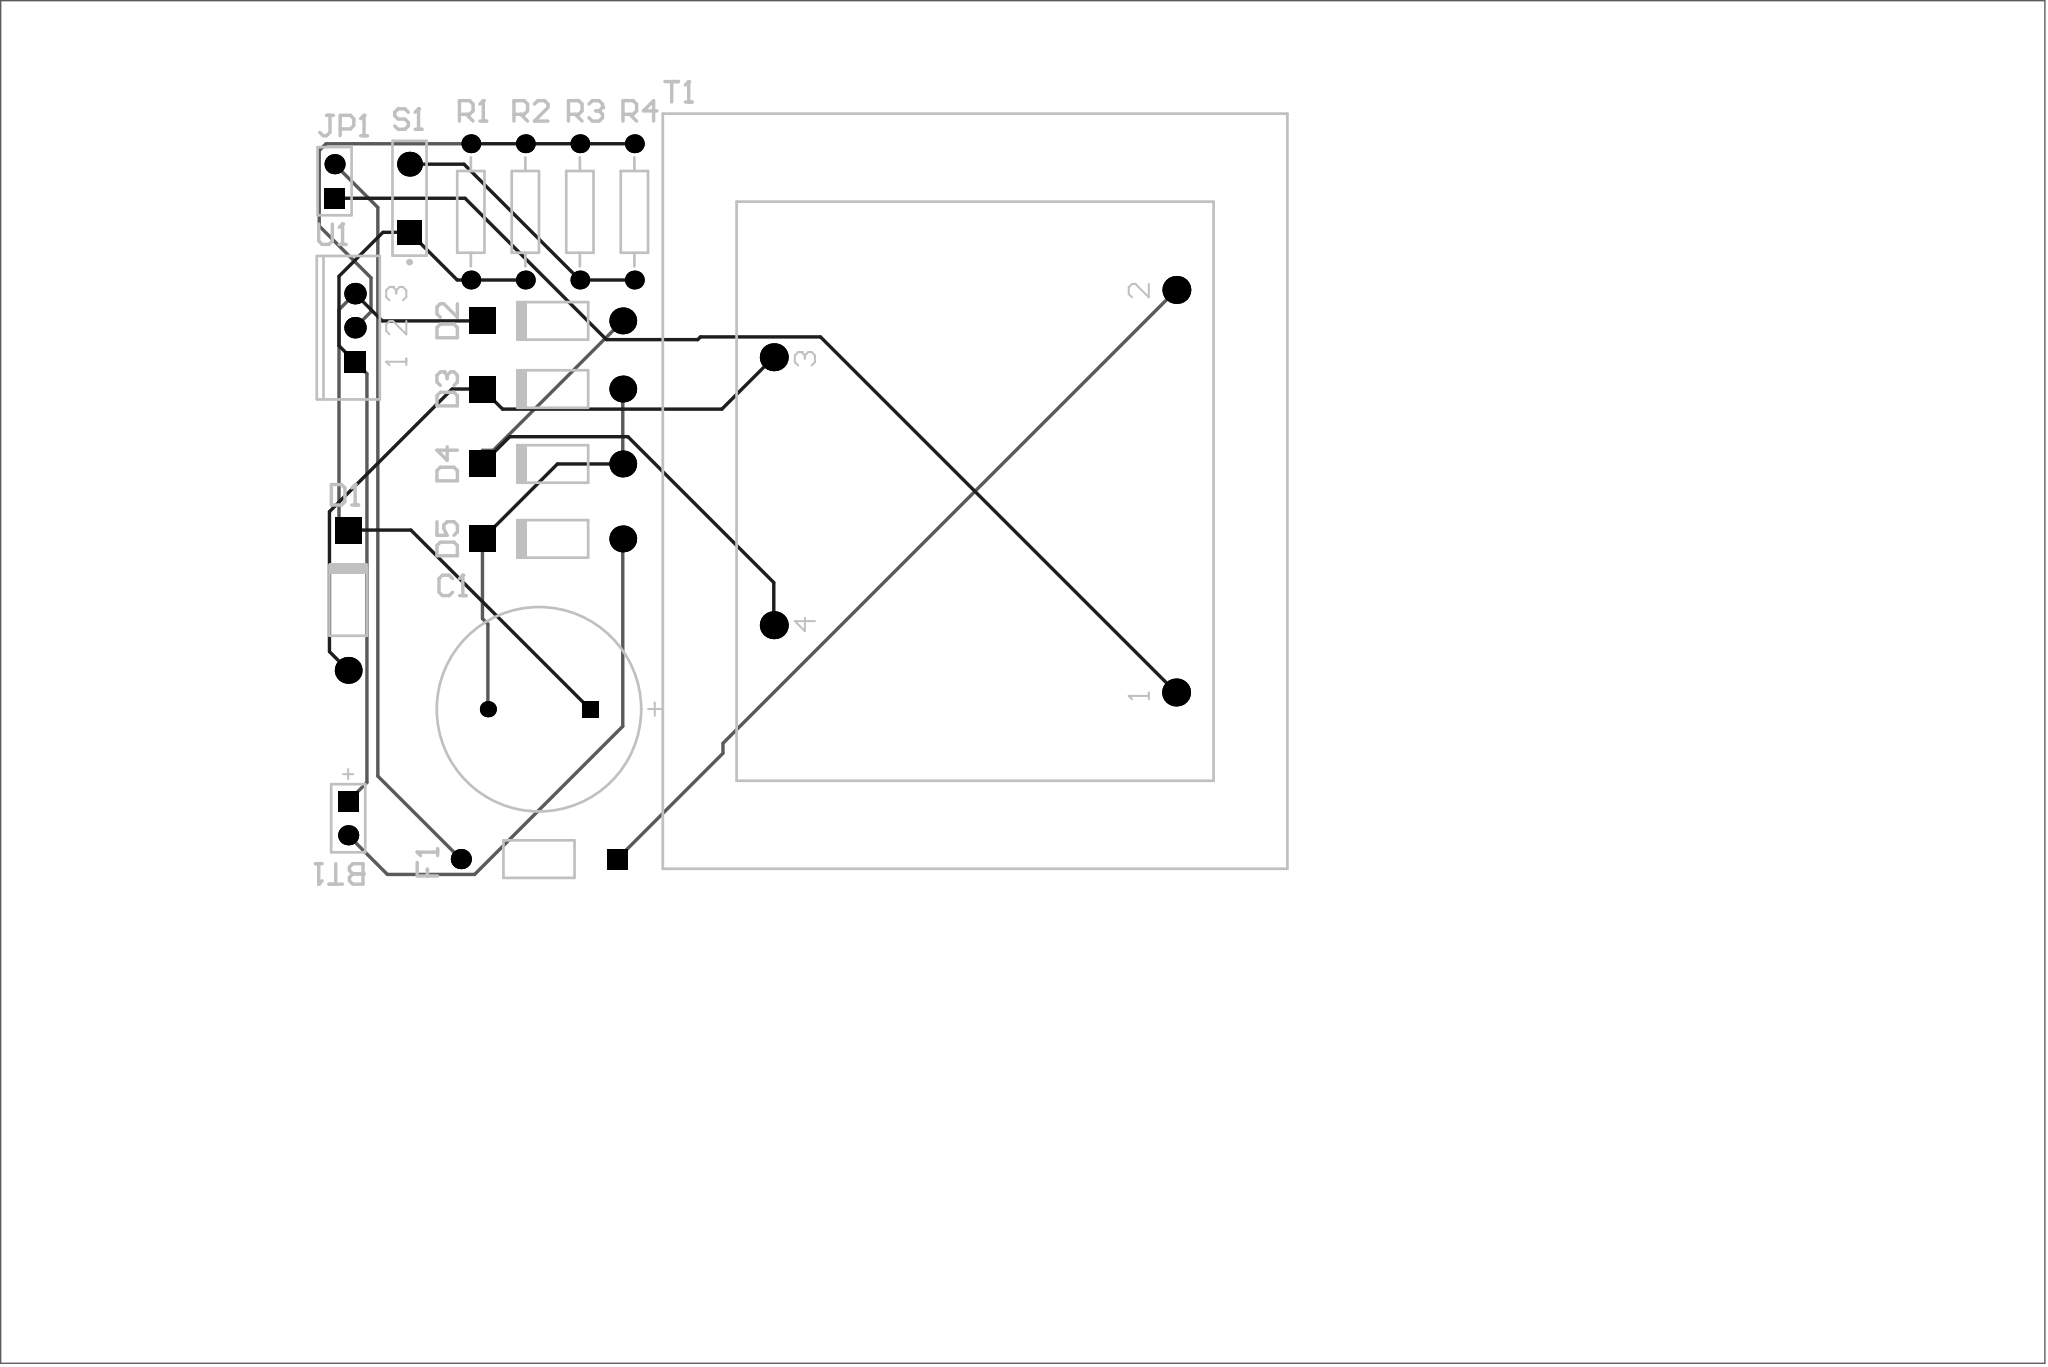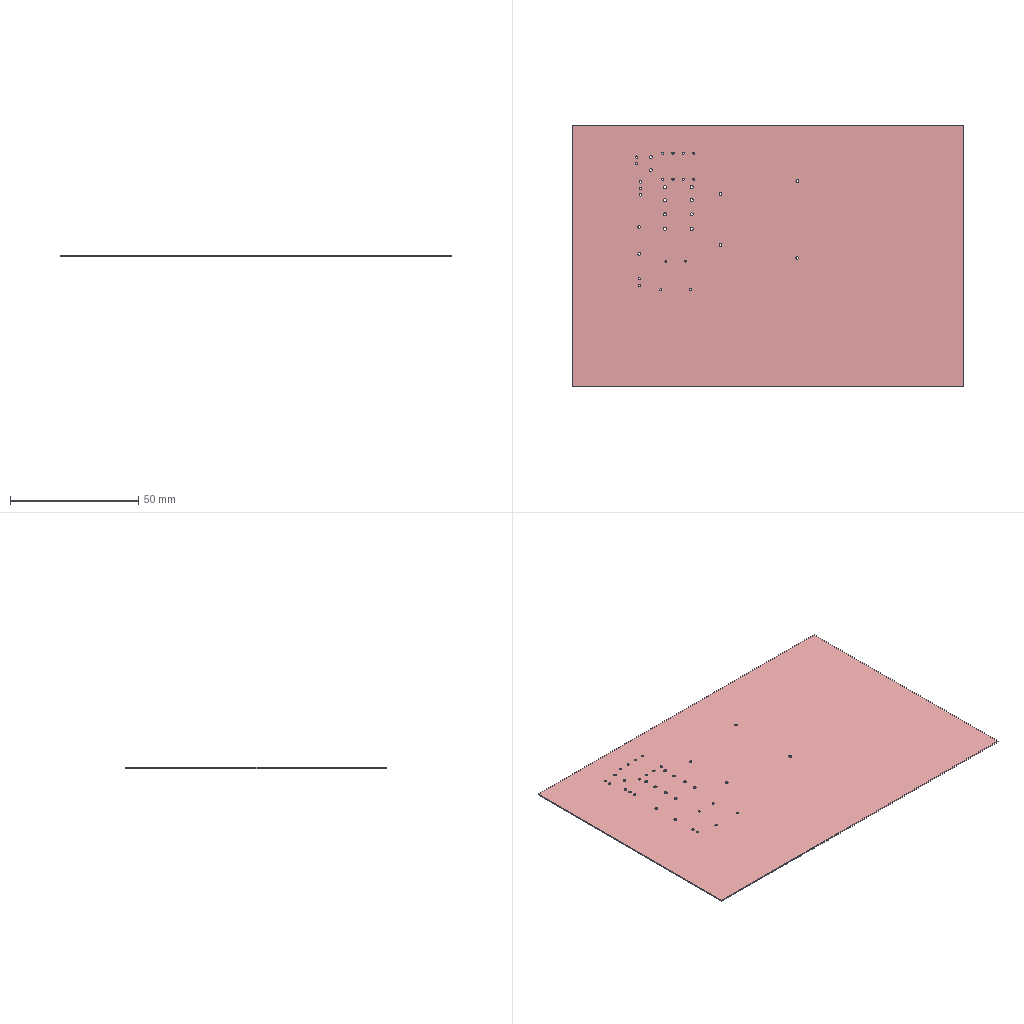Circuit board layout | Altium Designer | box 152.4 x 101.6 x 0.4 mm
Layer stack:
# Altium Designer layer stack of  (unit mm; dielectric type: 0 none, 1 core, 2 prepreg, 3 surface material)
index,name,kind,layer,copper_thickness_mm,dielectric_type,dielectric_thickness_mm,dielectric_material,dielectric_constant
0,Top Paste,other,,,,,,
1,Top Overlay,other,,,,,,
2,Top Solder,dielectric,,,3,0.0102,Solder Resist,3.5
3,Top Layer,copper,Top Layer,0.0356,,,,
4,Dielectric1,dielectric,,,0,0.32,FR-4,4.8
5,Bottom Layer,copper,Bottom Layer,0.0356,,,,
6,Bottom Solder,dielectric,,,3,0.0102,Solder Resist,3.5
7,Bottom Overlay,other,,,,,,
8,Bottom Paste,other,,,,,,
# drill layer pairs: low layer,high layer
drill_pair,Top Layer,Bottom Layer
Part placement:
Designator,Comment,Layer,Footprint,Center-X(mm),Center-Y(mm),Rotation
BT1,Battery,TopLayer,BAT-2,51.308,66.04,270
C1,Cap Pol1,TopLayer,RB7.6-15,65.532,74.168,0
D1,Diode 1N4007,TopLayer,DIO10.46-5.3x2.8,51.308,82.296,90
D2,Diode 1N4007,TopLayer,DIO10.46-5.3x2.8,66.548,103.124,180
D3,Diode 1N4007,TopLayer,DIO10.46-5.3x2.8,66.548,98.044,180
D4,Diode 1N4007,TopLayer,DIO10.46-5.3x2.8,66.548,92.456,180
D5,Diode 1N4007,TopLayer,DIO10.46-5.3x2.8,66.548,86.868,180
F1,Fuse 1,TopLayer,PIN-W2/E2.8,65.532,62.992,180
JP1,Header 2,TopLayer,HDR1X2,50.292,113.538,90
R1,Res2,TopLayer,AXIAL-0.4,60.452,111.252,90
R2,Res2,TopLayer,AXIAL-0.4,64.516,111.252,90
R3,Res2,TopLayer,AXIAL-0.4,68.58,111.252,90
R4,Res2,TopLayer,AXIAL-0.4,72.644,111.252,90
S1,SW-PB,TopLayer,SPST-2,55.88,112.268,90
T1,Trans Cupl,TopLayer,TRF_4,98.044,90.424,90
U1,LM317KC,TopLayer,KC03,51.816,102.616,90
Pad and via stacks:
# Altium Designer via and pad stacks of  (unit mm). Each distinct definition once, with the count of objects using it.
# via: kind,start_layer,end_layer,hole_mm,diameter_mm,mode(0 simple;1 top-mid-bottom;2 full stack),diameter_per_layer,count,example_net
# pad: kind,layer,hole_mm,hole_type(0 round;1 square;2 slot),plating,top_size,top_shape(1 round;2 rect;3 octagon;9 rounded rect),mid_size,bottom_size,mode,footprint,size_per_layer,count,example
pad,Multi-Layer,0.9,0,plated,1.5x1.5,2,1.5x1.5,1.5x1.5,0,BAT-2,,1,BT1.1
pad,Multi-Layer,0.9,0,plated,1.5x1.5,1,1.5x1.5,1.5x1.5,0,BAT-2,,1,BT1.2
pad,Multi-Layer,1.2,0,plated,2x2,1,2x2,2x2,0,DIO10.46-5.3x2.8,,5,D5.1
pad,Multi-Layer,1.2,0,plated,2x2,2,2x2,2x2,0,DIO10.46-5.3x2.8,,5,D5.2
pad,Multi-Layer,1.1,0,plated,1.85x1.85,2,1.85x1.85,1.85x1.85,0,SPST-2,,1,S1.1
pad,Multi-Layer,1.1,0,plated,1.85x1.85,1,1.85x1.85,1.85x1.85,0,SPST-2,,1,S1.2
pad,Multi-Layer,0.9,0,plated,1.5x1.5,2,1.5x1.5,1.5x1.5,0,PIN-W2/E2.8,,1,F1.1
pad,Multi-Layer,0.9,0,plated,1.5x1.5,1,1.5x1.5,1.5x1.5,0,PIN-W2/E2.8,,1,F1.2
pad,Multi-Layer,0.85,0,plated,1.4x1.4,1,1.4x1.4,1.4x1.4,0,AXIAL-0.4,,8,R1.2
pad,Multi-Layer,0.7,0,plated,1.2x1.2,2,1.2x1.2,1.2x1.2,0,RB7.6-15,,1,C1.1
pad,Multi-Layer,0.7,0,plated,1.2x1.2,1,1.2x1.2,1.2x1.2,0,RB7.6-15,,1,C1.2
pad,Multi-Layer,1.067,0,plated,2.083x2.083,1,2.083x2.083,2.083x2.083,0,TRF_4,,4,T1.4
pad,Multi-Layer,0.9,0,plated,1.5x1.5,1,1.5x1.5,1.5x1.5,0,HDR1X2,,1,JP1.2
pad,Multi-Layer,0.9,0,plated,1.5x1.5,2,1.5x1.5,1.5x1.5,0,HDR1X2,,1,JP1.1
pad,Multi-Layer,1,0,plated,1.6x1.6,1,1.6x1.6,1.6x1.6,0,KC03,,2,U1.3
pad,Multi-Layer,1,0,plated,1.6x1.6,2,1.6x1.6,1.6x1.6,0,KC03,,1,U1.1
Design rules, without the lines most boards share:
# Altium Designer design rules of  (exported by Altium Designer, unit mm)
# columns: name | kind | enabled | priority | scope1 | scope2 | descriptor | typed fields (field=value)
HoleToHoleClearance | 52 | enabled | 1 | All | All | Hole To Hole Clearance (Gap=10mil) (All),(All) | gap=0.254
DiffPairsRouting | 51 | enabled | 1 | All | All | Differential Pairs Uncoupled Length using the Gap Constraints (Min=10mil) (Max=10mil) (Prefered=10mil)  and Width Constraints (Min=15mil) (Max=15mil) (Prefered=15mil) (All) |
Clearance | 0 | enabled | 1 | All | All | Clearance Constraint (Gap=10mil) (All),(All) | gap=0.254
Width_1 | 2 | enabled | 1 | All | All | Width Constraint (Min=10mil) (Max=10mil) (Preferred=10mil) (All) |
RoutingCorners | 10 | enabled | 1 | All | All | Routing Corners (Style=Round) (Min Setback=100mil) (Max Setback=100mil) (All) |
RoutingVias | 11 | enabled | 1 | All | All | Routing Via (MinHoleWidth=28mil) (MaxHoleWidth=28mil) (PreferredHoleWidth=28mil) (MinWidth=50mil) (MaxWidth=50mil) (PreferedWidth=50mil) (All) | via_min_hole=0.7112 via_max_hole=0.7112 via_preferred_diameter=1.27 via_preferred_hole=0.7112
FanoutControl | 49 | enabled | 1 | All | All | Fanout Control Rule ( (All) ) |
PlaneConnect | 6 | enabled | 1 | All | All | Power Plane Connect Rule(Relief Connect )(Expansion=20mil) (Conductor Width=10mil) (Air Gap=10mil) (Entries=4) (All) | relief_conductor_width=0.254 relief_entries=4 relief_expansion=0.508
PolygonConnect | 20 | enabled | 1 | All | All | Polygon Connect Rule(Relief Connect )(Conductor Width=10mil) (Relief Angle=90 Angle) (Entries=4) (Air Gap Width=10mil) (All),(All) | connect_style(0=relief,1=direct,2=none)=0 relief_conductor_width=0.254 relief_entries=4
PasteMaskExpansion | 14 | enabled | 1 | All | All | Paste Mask Expansion (Expansion =0mil) (All) | expansion=0
SolderMaskExpansion | 13 | enabled | 1 | All | All | Solder Mask Expansion (Expansion =4mil) (All) | expansion=0.1016
TestPointUsage | 44 | enabled | 1 | All | All | Fabrication Testpoint Usage (Valid =One Required, Allow multiple per net=No) (All) |
Testpoint | 43 | enabled | 1 | All | All | Fabrication Testpoint Style (Under Component=Yes) (All) |